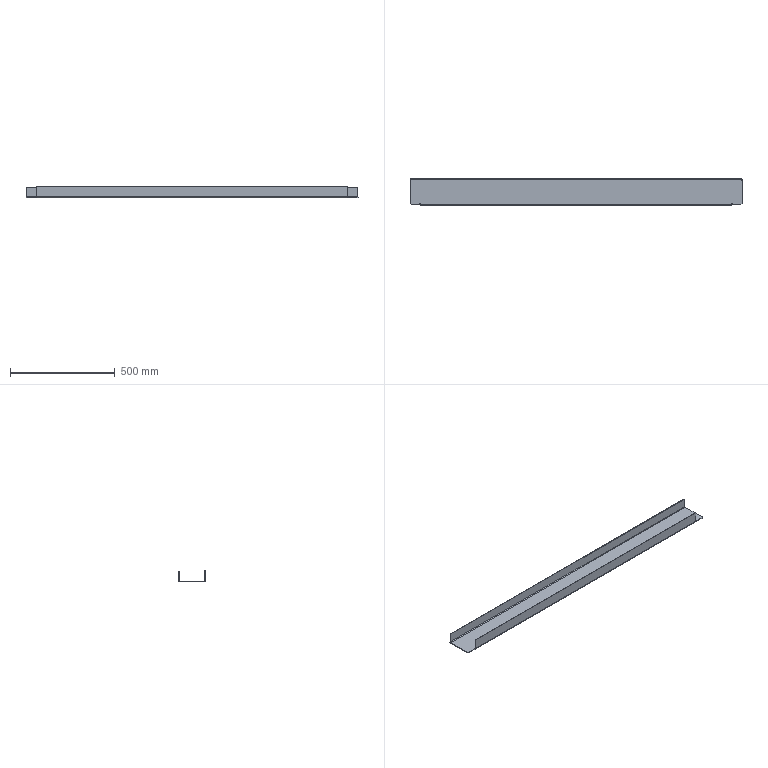Part | STEP file | SYL_0392D6J1SYL0380DJ100-794406 | 1 solid | 40 faces | box 1586 x 127 x 55 mm | volume 1040042 mm3 | plane 34 | cylinder 6 | commonest cylinder face diameters 6 x2 8 x2 12 x2
STEP:
#1=CARTESIAN_POINT('',(-744.,-57.5,3.));
#2=VERTEX_POINT('',#1);
#3=CARTESIAN_POINT('',(-744.,-57.5,0.));
#4=VERTEX_POINT('',#3);
#5=CARTESIAN_POINT('',(-744.,-57.5,0.));
#6=DIRECTION('',(0.,0.,-1.));
#7=VECTOR('',#6,1000.);
#8=LINE('',#5,#7);
#9=EDGE_CURVE('',#2,#4,#8,.T.);
#10=ORIENTED_EDGE('',*,*,#9,.F.);
#11=CARTESIAN_POINT('',(-745.5,-57.5,3.));
#12=VERTEX_POINT('',#11);
#13=CARTESIAN_POINT('',(0.,-57.5,3.));
#14=DIRECTION('',(-1.,0.,0.));
#15=VECTOR('',#14,1000.);
#16=LINE('',#13,#15);
#17=EDGE_CURVE('',#2,#12,#16,.T.);
#18=ORIENTED_EDGE('',*,*,#17,.T.);
#19=CARTESIAN_POINT('',(-745.5,-57.5,0.));
#20=VERTEX_POINT('',#19);
#21=CARTESIAN_POINT('',(-745.5,-57.5,0.));
#22=DIRECTION('',(0.,0.,-1.));
#23=VECTOR('',#22,1000.);
#24=LINE('',#21,#23);
#25=EDGE_CURVE('',#12,#20,#24,.T.);
#26=ORIENTED_EDGE('',*,*,#25,.T.);
#27=CARTESIAN_POINT('',(0.,-57.5,0.));
#28=DIRECTION('',(-1.,0.,0.));
#29=VECTOR('',#28,1000.);
#30=LINE('',#27,#29);
#31=EDGE_CURVE('',#4,#20,#30,.T.);
#32=ORIENTED_EDGE('',*,*,#31,.F.);
#33=EDGE_LOOP('',(#10,#18,#26,#32));
#34=FACE_OUTER_BOUND('',#33,.T.);
#35=CARTESIAN_POINT('',(0.,-57.5,0.));
#36=DIRECTION('',(0.,1.,0.));
#37=DIRECTION('',(-1.,0.,0.));
#38=AXIS2_PLACEMENT_3D('',#35,#36,#37);
#39=PLANE('',#38);
#40=ADVANCED_FACE('',(#34),#39,.F.);
#41=ORIENTED_EDGE('',*,*,#25,.F.);
#42=CARTESIAN_POINT('',(-745.5,-62.,3.));
#43=VERTEX_POINT('',#42);
#44=CARTESIAN_POINT('',(-745.5,0.,3.));
#45=DIRECTION('',(0.,-1.,0.));
#46=VECTOR('',#45,1000.);
#47=LINE('',#44,#46);
#48=EDGE_CURVE('',#12,#43,#47,.T.);
#49=ORIENTED_EDGE('',*,*,#48,.T.);
#50=CARTESIAN_POINT('',(-745.5,-62.,0.));
#51=VERTEX_POINT('',#50);
#52=CARTESIAN_POINT('',(-745.5,-62.,0.));
#53=DIRECTION('',(0.,0.,-1.));
#54=VECTOR('',#53,1000.);
#55=LINE('',#52,#54);
#56=EDGE_CURVE('',#43,#51,#55,.T.);
#57=ORIENTED_EDGE('',*,*,#56,.T.);
#58=CARTESIAN_POINT('',(-745.5,0.,0.));
#59=DIRECTION('',(0.,-1.,0.));
#60=VECTOR('',#59,1000.);
#61=LINE('',#58,#60);
#62=EDGE_CURVE('',#20,#51,#61,.T.);
#63=ORIENTED_EDGE('',*,*,#62,.F.);
#64=EDGE_LOOP('',(#41,#49,#57,#63));
#65=FACE_OUTER_BOUND('',#64,.T.);
#66=CARTESIAN_POINT('',(-745.5,0.,0.));
#67=DIRECTION('',(-1.,0.,0.));
#68=DIRECTION('',(0.,-1.,0.));
#69=AXIS2_PLACEMENT_3D('',#66,#67,#68);
#70=PLANE('',#69);
#71=ADVANCED_FACE('',(#65),#70,.F.);
#72=ORIENTED_EDGE('',*,*,#56,.F.);
#73=CARTESIAN_POINT('',(-788.,-62.,3.));
#74=VERTEX_POINT('',#73);
#75=CARTESIAN_POINT('',(0.,-62.,3.));
#76=DIRECTION('',(1.,0.,0.));
#77=VECTOR('',#76,1000.);
#78=LINE('',#75,#77);
#79=EDGE_CURVE('',#74,#43,#78,.T.);
#80=ORIENTED_EDGE('',*,*,#79,.F.);
#81=CARTESIAN_POINT('',(-788.,-62.,0.));
#82=VERTEX_POINT('',#81);
#83=CARTESIAN_POINT('',(-788.,-62.,0.));
#84=DIRECTION('',(0.,0.,-1.));
#85=VECTOR('',#84,1000.);
#86=LINE('',#83,#85);
#87=EDGE_CURVE('',#74,#82,#86,.T.);
#88=ORIENTED_EDGE('',*,*,#87,.T.);
#89=CARTESIAN_POINT('',(-788.,-62.,0.));
#90=DIRECTION('',(1.,0.,0.));
#91=VECTOR('',#90,1000.);
#92=LINE('',#89,#91);
#93=EDGE_CURVE('',#82,#51,#92,.T.);
#94=ORIENTED_EDGE('',*,*,#93,.T.);
#95=EDGE_LOOP('',(#72,#80,#88,#94));
#96=FACE_OUTER_BOUND('',#95,.T.);
#97=CARTESIAN_POINT('',(-788.,-62.,0.));
#98=DIRECTION('',(0.,-1.,0.));
#99=DIRECTION('',(1.,0.,0.));
#100=AXIS2_PLACEMENT_3D('',#97,#98,#99);
#101=PLANE('',#100);
#102=ADVANCED_FACE('',(#96),#101,.T.);
#103=ORIENTED_EDGE('',*,*,#87,.F.);
#104=CARTESIAN_POINT('',(-793.,-57.,3.));
#105=VERTEX_POINT('',#104);
#106=CARTESIAN_POINT('',(-788.,-62.,3.));
#107=DIRECTION('',(-0.7071,0.7071,0.));
#108=VECTOR('',#107,1000.);
#109=LINE('',#106,#108);
#110=EDGE_CURVE('',#74,#105,#109,.T.);
#111=ORIENTED_EDGE('',*,*,#110,.T.);
#112=CARTESIAN_POINT('',(-793.,-57.,0.));
#113=VERTEX_POINT('',#112);
#114=CARTESIAN_POINT('',(-793.,-57.,0.));
#115=DIRECTION('',(0.,0.,-1.));
#116=VECTOR('',#115,1000.);
#117=LINE('',#114,#116);
#118=EDGE_CURVE('',#105,#113,#117,.T.);
#119=ORIENTED_EDGE('',*,*,#118,.T.);
#120=CARTESIAN_POINT('',(-788.,-62.,0.));
#121=DIRECTION('',(-0.7071,0.7071,0.));
#122=VECTOR('',#121,1000.);
#123=LINE('',#120,#122);
#124=EDGE_CURVE('',#82,#113,#123,.T.);
#125=ORIENTED_EDGE('',*,*,#124,.F.);
#126=EDGE_LOOP('',(#103,#111,#119,#125));
#127=FACE_OUTER_BOUND('',#126,.T.);
#128=CARTESIAN_POINT('',(-788.,-62.,0.));
#129=DIRECTION('',(0.7071,0.7071,0.));
#130=DIRECTION('',(-0.7071,0.7071,0.));
#131=AXIS2_PLACEMENT_3D('',#128,#129,#130);
#132=PLANE('',#131);
#133=ADVANCED_FACE('',(#127),#132,.F.);
#134=ORIENTED_EDGE('',*,*,#118,.F.);
#135=CARTESIAN_POINT('',(-793.,58.,3.));
#136=VERTEX_POINT('',#135);
#137=CARTESIAN_POINT('',(-793.,0.,3.));
#138=DIRECTION('',(0.,-1.,0.));
#139=VECTOR('',#138,1000.);
#140=LINE('',#137,#139);
#141=EDGE_CURVE('',#136,#105,#140,.T.);
#142=ORIENTED_EDGE('',*,*,#141,.F.);
#143=CARTESIAN_POINT('',(-793.,58.,0.));
#144=VERTEX_POINT('',#143);
#145=CARTESIAN_POINT('',(-793.,58.,0.));
#146=DIRECTION('',(0.,0.,-1.));
#147=VECTOR('',#146,1000.);
#148=LINE('',#145,#147);
#149=EDGE_CURVE('',#136,#144,#148,.T.);
#150=ORIENTED_EDGE('',*,*,#149,.T.);
#151=CARTESIAN_POINT('',(-793.,58.,0.));
#152=DIRECTION('',(0.,-1.,0.));
#153=VECTOR('',#152,1000.);
#154=LINE('',#151,#153);
#155=EDGE_CURVE('',#144,#113,#154,.T.);
#156=ORIENTED_EDGE('',*,*,#155,.T.);
#157=EDGE_LOOP('',(#134,#142,#150,#156));
#158=FACE_OUTER_BOUND('',#157,.T.);
#159=CARTESIAN_POINT('',(-793.,58.,0.));
#160=DIRECTION('',(-1.,0.,0.));
#161=DIRECTION('',(0.,-1.,0.));
#162=AXIS2_PLACEMENT_3D('',#159,#160,#161);
#163=PLANE('',#162);
#164=ADVANCED_FACE('',(#158),#163,.T.);
#165=ORIENTED_EDGE('',*,*,#149,.F.);
#166=CARTESIAN_POINT('',(-790.5,61.708,3.));
#167=VERTEX_POINT('',#166);
#168=CARTESIAN_POINT('',(-789.,58.,3.));
#169=DIRECTION('',(0.,0.,-1.));
#170=DIRECTION('',(-1.,0.,0.));
#171=AXIS2_PLACEMENT_3D('',#168,#169,#170);
#172=CIRCLE('',#171,4.);
#173=EDGE_CURVE('',#136,#167,#172,.T.);
#174=ORIENTED_EDGE('',*,*,#173,.T.);
#175=CARTESIAN_POINT('',(-790.5,61.708,0.));
#176=VERTEX_POINT('',#175);
#177=CARTESIAN_POINT('',(-790.5,61.708,0.));
#178=DIRECTION('',(0.,0.,-1.));
#179=VECTOR('',#178,1000.);
#180=LINE('',#177,#179);
#181=EDGE_CURVE('',#167,#176,#180,.T.);
#182=ORIENTED_EDGE('',*,*,#181,.T.);
#183=CARTESIAN_POINT('',(-789.,58.,0.));
#184=DIRECTION('',(0.,0.,-1.));
#185=DIRECTION('',(-1.,0.,0.));
#186=AXIS2_PLACEMENT_3D('',#183,#184,#185);
#187=CIRCLE('',#186,4.);
#188=EDGE_CURVE('',#144,#176,#187,.T.);
#189=ORIENTED_EDGE('',*,*,#188,.F.);
#190=EDGE_LOOP('',(#165,#174,#182,#189));
#191=FACE_OUTER_BOUND('',#190,.T.);
#192=CARTESIAN_POINT('',(-789.,58.,0.));
#193=DIRECTION('',(0.,0.,1.));
#194=DIRECTION('',(1.,0.,0.));
#195=AXIS2_PLACEMENT_3D('',#192,#193,#194);
#196=CYLINDRICAL_SURFACE('',#195,4.);
#197=ADVANCED_FACE('',(#191),#196,.T.);
#198=ORIENTED_EDGE('',*,*,#181,.F.);
#199=CARTESIAN_POINT('',(-790.5,54.5,3.));
#200=VERTEX_POINT('',#199);
#201=CARTESIAN_POINT('',(-790.5,0.,3.));
#202=DIRECTION('',(0.,-1.,0.));
#203=VECTOR('',#202,1000.);
#204=LINE('',#201,#203);
#205=EDGE_CURVE('',#167,#200,#204,.T.);
#206=ORIENTED_EDGE('',*,*,#205,.T.);
#207=CARTESIAN_POINT('',(-790.5,54.5,0.));
#208=VERTEX_POINT('',#207);
#209=CARTESIAN_POINT('',(-790.5,54.5,0.));
#210=DIRECTION('',(0.,0.,-1.));
#211=VECTOR('',#210,1000.);
#212=LINE('',#209,#211);
#213=EDGE_CURVE('',#200,#208,#212,.T.);
#214=ORIENTED_EDGE('',*,*,#213,.T.);
#215=CARTESIAN_POINT('',(-790.5,0.,0.));
#216=DIRECTION('',(0.,-1.,0.));
#217=VECTOR('',#216,1000.);
#218=LINE('',#215,#217);
#219=EDGE_CURVE('',#176,#208,#218,.T.);
#220=ORIENTED_EDGE('',*,*,#219,.F.);
#221=EDGE_LOOP('',(#198,#206,#214,#220));
#222=FACE_OUTER_BOUND('',#221,.T.);
#223=CARTESIAN_POINT('',(-790.5,0.,0.));
#224=DIRECTION('',(-1.,0.,0.));
#225=DIRECTION('',(0.,-1.,0.));
#226=AXIS2_PLACEMENT_3D('',#223,#224,#225);
#227=PLANE('',#226);
#228=ADVANCED_FACE('',(#222),#227,.F.);
#229=ORIENTED_EDGE('',*,*,#213,.F.);
#230=CARTESIAN_POINT('',(-789.,54.5,3.));
#231=VERTEX_POINT('',#230);
#232=CARTESIAN_POINT('',(0.,54.5,3.));
#233=DIRECTION('',(1.,0.,0.));
#234=VECTOR('',#233,1000.);
#235=LINE('',#232,#234);
#236=EDGE_CURVE('',#200,#231,#235,.T.);
#237=ORIENTED_EDGE('',*,*,#236,.T.);
#238=CARTESIAN_POINT('',(-789.,54.5,0.));
#239=VERTEX_POINT('',#238);
#240=CARTESIAN_POINT('',(-789.,54.5,0.));
#241=DIRECTION('',(0.,0.,-1.));
#242=VECTOR('',#241,1000.);
#243=LINE('',#240,#242);
#244=EDGE_CURVE('',#231,#239,#243,.T.);
#245=ORIENTED_EDGE('',*,*,#244,.T.);
#246=CARTESIAN_POINT('',(0.,54.5,0.));
#247=DIRECTION('',(1.,0.,0.));
#248=VECTOR('',#247,1000.);
#249=LINE('',#246,#248);
#250=EDGE_CURVE('',#208,#239,#249,.T.);
#251=ORIENTED_EDGE('',*,*,#250,.F.);
#252=EDGE_LOOP('',(#229,#237,#245,#251));
#253=FACE_OUTER_BOUND('',#252,.T.);
#254=CARTESIAN_POINT('',(0.,54.5,0.));
#255=DIRECTION('',(0.,-1.,0.));
#256=DIRECTION('',(1.,0.,0.));
#257=AXIS2_PLACEMENT_3D('',#254,#255,#256);
#258=PLANE('',#257);
#259=ADVANCED_FACE('',(#253),#258,.F.);
#260=ORIENTED_EDGE('',*,*,#244,.F.);
#261=CARTESIAN_POINT('',(-789.,56.,3.));
#262=VERTEX_POINT('',#261);
#263=CARTESIAN_POINT('',(-789.,0.,3.));
#264=DIRECTION('',(0.,1.,0.));
#265=VECTOR('',#264,1000.);
#266=LINE('',#263,#265);
#267=EDGE_CURVE('',#231,#262,#266,.T.);
#268=ORIENTED_EDGE('',*,*,#267,.T.);
#269=CARTESIAN_POINT('',(-789.,56.,0.));
#270=VERTEX_POINT('',#269);
#271=CARTESIAN_POINT('',(-789.,56.,0.));
#272=DIRECTION('',(0.,0.,-1.));
#273=VECTOR('',#272,1000.);
#274=LINE('',#271,#273);
#275=EDGE_CURVE('',#262,#270,#274,.T.);
#276=ORIENTED_EDGE('',*,*,#275,.T.);
#277=CARTESIAN_POINT('',(-789.,0.,0.));
#278=DIRECTION('',(0.,1.,0.));
#279=VECTOR('',#278,1000.);
#280=LINE('',#277,#279);
#281=EDGE_CURVE('',#239,#270,#280,.T.);
#282=ORIENTED_EDGE('',*,*,#281,.F.);
#283=EDGE_LOOP('',(#260,#268,#276,#282));
#284=FACE_OUTER_BOUND('',#283,.T.);
#285=CARTESIAN_POINT('',(-789.,0.,0.));
#286=DIRECTION('',(1.,0.,0.));
#287=DIRECTION('',(0.,1.,0.));
#288=AXIS2_PLACEMENT_3D('',#285,#286,#287);
#289=PLANE('',#288);
#290=ADVANCED_FACE('',(#284),#289,.F.);
#291=ORIENTED_EDGE('',*,*,#275,.F.);
#292=CARTESIAN_POINT('',(-789.,59.,6.));
#293=VERTEX_POINT('',#292);
#294=CARTESIAN_POINT('',(-789.,56.,6.));
#295=DIRECTION('',(-1.,0.,0.));
#296=DIRECTION('',(0.,0.,1.));
#297=AXIS2_PLACEMENT_3D('',#294,#295,#296);
#298=CIRCLE('',#297,3.);
#299=EDGE_CURVE('',#293,#262,#298,.T.);
#300=ORIENTED_EDGE('',*,*,#299,.F.);
#301=CARTESIAN_POINT('',(-789.,62.,6.));
#302=VERTEX_POINT('',#301);
#303=CARTESIAN_POINT('',(-789.,62.,6.));
#304=DIRECTION('',(0.,1.,0.));
#305=VECTOR('',#304,1000.);
#306=LINE('',#303,#305);
#307=EDGE_CURVE('',#293,#302,#306,.T.);
#308=ORIENTED_EDGE('',*,*,#307,.T.);
#309=CARTESIAN_POINT('',(-789.,56.,6.));
#310=DIRECTION('',(-1.,0.,0.));
#311=DIRECTION('',(0.,1.,0.));
#312=AXIS2_PLACEMENT_3D('',#309,#310,#311);
#313=CIRCLE('',#312,6.);
#314=EDGE_CURVE('',#302,#270,#313,.T.);
#315=ORIENTED_EDGE('',*,*,#314,.T.);
#316=EDGE_LOOP('',(#291,#300,#308,#315));
#317=FACE_OUTER_BOUND('',#316,.T.);
#318=CARTESIAN_POINT('',(-789.,56.,6.));
#319=DIRECTION('',(1.,0.,0.));
#320=DIRECTION('',(0.,0.,-1.));
#321=AXIS2_PLACEMENT_3D('',#318,#319,#320);
#322=PLANE('',#321);
#323=ADVANCED_FACE('',(#317),#322,.F.);
#324=ORIENTED_EDGE('',*,*,#307,.F.);
#325=CARTESIAN_POINT('',(-789.,59.,50.));
#326=VERTEX_POINT('',#325);
#327=CARTESIAN_POINT('',(-789.,59.,0.));
#328=DIRECTION('',(0.,0.,1.));
#329=VECTOR('',#328,1000.);
#330=LINE('',#327,#329);
#331=EDGE_CURVE('',#293,#326,#330,.T.);
#332=ORIENTED_EDGE('',*,*,#331,.T.);
#333=CARTESIAN_POINT('',(-789.,62.,50.));
#334=VERTEX_POINT('',#333);
#335=CARTESIAN_POINT('',(-789.,62.,50.));
#336=DIRECTION('',(0.,1.,0.));
#337=VECTOR('',#336,1000.);
#338=LINE('',#335,#337);
#339=EDGE_CURVE('',#326,#334,#338,.T.);
#340=ORIENTED_EDGE('',*,*,#339,.T.);
#341=CARTESIAN_POINT('',(-789.,62.,6.));
#342=DIRECTION('',(0.,0.,1.));
#343=VECTOR('',#342,1000.);
#344=LINE('',#341,#343);
#345=EDGE_CURVE('',#302,#334,#344,.T.);
#346=ORIENTED_EDGE('',*,*,#345,.F.);
#347=EDGE_LOOP('',(#324,#332,#340,#346));
#348=FACE_OUTER_BOUND('',#347,.T.);
#349=CARTESIAN_POINT('',(-789.,62.,6.));
#350=DIRECTION('',(-1.,0.,0.));
#351=DIRECTION('',(0.,0.,1.));
#352=AXIS2_PLACEMENT_3D('',#349,#350,#351);
#353=PLANE('',#352);
#354=ADVANCED_FACE('',(#348),#353,.T.);
#355=ORIENTED_EDGE('',*,*,#339,.F.);
#356=CARTESIAN_POINT('',(789.,59.,50.));
#357=VERTEX_POINT('',#356);
#358=CARTESIAN_POINT('',(-789.,59.,50.));
#359=DIRECTION('',(1.,0.,0.));
#360=VECTOR('',#359,1000.);
#361=LINE('',#358,#360);
#362=EDGE_CURVE('',#326,#357,#361,.T.);
#363=ORIENTED_EDGE('',*,*,#362,.T.);
#364=CARTESIAN_POINT('',(789.,62.,50.));
#365=VERTEX_POINT('',#364);
#366=CARTESIAN_POINT('',(789.,62.,50.));
#367=DIRECTION('',(0.,1.,0.));
#368=VECTOR('',#367,1000.);
#369=LINE('',#366,#368);
#370=EDGE_CURVE('',#357,#365,#369,.T.);
#371=ORIENTED_EDGE('',*,*,#370,.T.);
#372=CARTESIAN_POINT('',(-789.,62.,50.));
#373=DIRECTION('',(1.,0.,0.));
#374=VECTOR('',#373,1000.);
#375=LINE('',#372,#374);
#376=EDGE_CURVE('',#334,#365,#375,.T.);
#377=ORIENTED_EDGE('',*,*,#376,.F.);
#378=EDGE_LOOP('',(#355,#363,#371,#377));
#379=FACE_OUTER_BOUND('',#378,.T.);
#380=CARTESIAN_POINT('',(-789.,62.,50.));
#381=DIRECTION('',(0.,0.,1.));
#382=DIRECTION('',(1.,0.,0.));
#383=AXIS2_PLACEMENT_3D('',#380,#381,#382);
#384=PLANE('',#383);
#385=ADVANCED_FACE('',(#379),#384,.T.);
#386=ORIENTED_EDGE('',*,*,#370,.F.);
#387=CARTESIAN_POINT('',(789.,59.,6.));
#388=VERTEX_POINT('',#387);
#389=CARTESIAN_POINT('',(789.,59.,0.));
#390=DIRECTION('',(0.,0.,-1.));
#391=VECTOR('',#390,1000.);
#392=LINE('',#389,#391);
#393=EDGE_CURVE('',#357,#388,#392,.T.);
#394=ORIENTED_EDGE('',*,*,#393,.T.);
#395=CARTESIAN_POINT('',(789.,62.,6.));
#396=VERTEX_POINT('',#395);
#397=CARTESIAN_POINT('',(789.,62.,6.));
#398=DIRECTION('',(0.,1.,0.));
#399=VECTOR('',#398,1000.);
#400=LINE('',#397,#399);
#401=EDGE_CURVE('',#388,#396,#400,.T.);
#402=ORIENTED_EDGE('',*,*,#401,.T.);
#403=CARTESIAN_POINT('',(789.,62.,50.));
#404=DIRECTION('',(0.,0.,-1.));
#405=VECTOR('',#404,1000.);
#406=LINE('',#403,#405);
#407=EDGE_CURVE('',#365,#396,#406,.T.);
#408=ORIENTED_EDGE('',*,*,#407,.F.);
#409=EDGE_LOOP('',(#386,#394,#402,#408));
#410=FACE_OUTER_BOUND('',#409,.T.);
#411=CARTESIAN_POINT('',(789.,62.,50.));
#412=DIRECTION('',(1.,0.,0.));
#413=DIRECTION('',(0.,0.,-1.));
#414=AXIS2_PLACEMENT_3D('',#411,#412,#413);
#415=PLANE('',#414);
#416=ADVANCED_FACE('',(#410),#415,.T.);
#417=ORIENTED_EDGE('',*,*,#401,.F.);
#418=CARTESIAN_POINT('',(789.,56.,3.));
#419=VERTEX_POINT('',#418);
#420=CARTESIAN_POINT('',(789.,56.,6.));
#421=DIRECTION('',(1.,0.,0.));
#422=DIRECTION('',(0.,0.,1.));
#423=AXIS2_PLACEMENT_3D('',#420,#421,#422);
#424=CIRCLE('',#423,3.);
#425=EDGE_CURVE('',#419,#388,#424,.T.);
#426=ORIENTED_EDGE('',*,*,#425,.F.);
#427=CARTESIAN_POINT('',(789.,56.,0.));
#428=VERTEX_POINT('',#427);
#429=CARTESIAN_POINT('',(789.,56.,0.));
#430=DIRECTION('',(0.,0.,-1.));
#431=VECTOR('',#430,1000.);
#432=LINE('',#429,#431);
#433=EDGE_CURVE('',#419,#428,#432,.T.);
#434=ORIENTED_EDGE('',*,*,#433,.T.);
#435=CARTESIAN_POINT('',(789.,56.,6.));
#436=DIRECTION('',(1.,0.,0.));
#437=DIRECTION('',(0.,0.,-1.));
#438=AXIS2_PLACEMENT_3D('',#435,#436,#437);
#439=CIRCLE('',#438,6.);
#440=EDGE_CURVE('',#428,#396,#439,.T.);
#441=ORIENTED_EDGE('',*,*,#440,.T.);
#442=EDGE_LOOP('',(#417,#426,#434,#441));
#443=FACE_OUTER_BOUND('',#442,.T.);
#444=CARTESIAN_POINT('',(789.,56.,6.));
#445=DIRECTION('',(-1.,0.,0.));
#446=DIRECTION('',(0.,0.,1.));
#447=AXIS2_PLACEMENT_3D('',#444,#445,#446);
#448=PLANE('',#447);
#449=ADVANCED_FACE('',(#443),#448,.F.);
#450=ORIENTED_EDGE('',*,*,#433,.F.);
#451=CARTESIAN_POINT('',(789.,54.5,3.));
#452=VERTEX_POINT('',#451);
#453=CARTESIAN_POINT('',(789.,0.,3.));
#454=DIRECTION('',(0.,-1.,0.));
#455=VECTOR('',#454,1000.);
#456=LINE('',#453,#455);
#457=EDGE_CURVE('',#419,#452,#456,.T.);
#458=ORIENTED_EDGE('',*,*,#457,.T.);
#459=CARTESIAN_POINT('',(789.,54.5,0.));
#460=VERTEX_POINT('',#459);
#461=CARTESIAN_POINT('',(789.,54.5,0.));
#462=DIRECTION('',(0.,0.,-1.));
#463=VECTOR('',#462,1000.);
#464=LINE('',#461,#463);
#465=EDGE_CURVE('',#452,#460,#464,.T.);
#466=ORIENTED_EDGE('',*,*,#465,.T.);
#467=CARTESIAN_POINT('',(789.,0.,0.));
#468=DIRECTION('',(0.,-1.,0.));
#469=VECTOR('',#468,1000.);
#470=LINE('',#467,#469);
#471=EDGE_CURVE('',#428,#460,#470,.T.);
#472=ORIENTED_EDGE('',*,*,#471,.F.);
#473=EDGE_LOOP('',(#450,#458,#466,#472));
#474=FACE_OUTER_BOUND('',#473,.T.);
#475=CARTESIAN_POINT('',(789.,0.,0.));
#476=DIRECTION('',(-1.,0.,0.));
#477=DIRECTION('',(0.,-1.,0.));
#478=AXIS2_PLACEMENT_3D('',#475,#476,#477);
#479=PLANE('',#478);
#480=ADVANCED_FACE('',(#474),#479,.F.);
#481=ORIENTED_EDGE('',*,*,#465,.F.);
#482=CARTESIAN_POINT('',(790.5,54.5,3.));
#483=VERTEX_POINT('',#482);
#484=CARTESIAN_POINT('',(0.,54.5,3.));
#485=DIRECTION('',(1.,0.,0.));
#486=VECTOR('',#485,1000.);
#487=LINE('',#484,#486);
#488=EDGE_CURVE('',#452,#483,#487,.T.);
#489=ORIENTED_EDGE('',*,*,#488,.T.);
#490=CARTESIAN_POINT('',(790.5,54.5,0.));
#491=VERTEX_POINT('',#490);
#492=CARTESIAN_POINT('',(790.5,54.5,0.));
#493=DIRECTION('',(0.,0.,-1.));
#494=VECTOR('',#493,1000.);
#495=LINE('',#492,#494);
#496=EDGE_CURVE('',#483,#491,#495,.T.);
#497=ORIENTED_EDGE('',*,*,#496,.T.);
#498=CARTESIAN_POINT('',(0.,54.5,0.));
#499=DIRECTION('',(1.,0.,0.));
#500=VECTOR('',#499,1000.);
#501=LINE('',#498,#500);
#502=EDGE_CURVE('',#460,#491,#501,.T.);
#503=ORIENTED_EDGE('',*,*,#502,.F.);
#504=EDGE_LOOP('',(#481,#489,#497,#503));
#505=FACE_OUTER_BOUND('',#504,.T.);
#506=CARTESIAN_POINT('',(0.,54.5,0.));
#507=DIRECTION('',(0.,-1.,0.));
#508=DIRECTION('',(1.,0.,0.));
#509=AXIS2_PLACEMENT_3D('',#506,#507,#508);
#510=PLANE('',#509);
#511=ADVANCED_FACE('',(#505),#510,.F.);
#512=ORIENTED_EDGE('',*,*,#496,.F.);
#513=CARTESIAN_POINT('',(790.5,61.708,3.));
#514=VERTEX_POINT('',#513);
#515=CARTESIAN_POINT('',(790.5,0.,3.));
#516=DIRECTION('',(0.,1.,0.));
#517=VECTOR('',#516,1000.);
#518=LINE('',#515,#517);
#519=EDGE_CURVE('',#483,#514,#518,.T.);
#520=ORIENTED_EDGE('',*,*,#519,.T.);
#521=CARTESIAN_POINT('',(790.5,61.708,0.));
#522=VERTEX_POINT('',#521);
#523=CARTESIAN_POINT('',(790.5,61.708,0.));
#524=DIRECTION('',(0.,0.,-1.));
#525=VECTOR('',#524,1000.);
#526=LINE('',#523,#525);
#527=EDGE_CURVE('',#514,#522,#526,.T.);
#528=ORIENTED_EDGE('',*,*,#527,.T.);
#529=CARTESIAN_POINT('',(790.5,0.,0.));
#530=DIRECTION('',(0.,1.,0.));
#531=VECTOR('',#530,1000.);
#532=LINE('',#529,#531);
#533=EDGE_CURVE('',#491,#522,#532,.T.);
#534=ORIENTED_EDGE('',*,*,#533,.F.);
#535=EDGE_LOOP('',(#512,#520,#528,#534));
#536=FACE_OUTER_BOUND('',#535,.T.);
#537=CARTESIAN_POINT('',(790.5,0.,0.));
#538=DIRECTION('',(1.,0.,0.));
#539=DIRECTION('',(0.,1.,0.));
#540=AXIS2_PLACEMENT_3D('',#537,#538,#539);
#541=PLANE('',#540);
#542=ADVANCED_FACE('',(#536),#541,.F.);
#543=ORIENTED_EDGE('',*,*,#527,.F.);
#544=CARTESIAN_POINT('',(793.,58.,3.));
#545=VERTEX_POINT('',#544);
#546=CARTESIAN_POINT('',(789.,58.,3.));
#547=DIRECTION('',(0.,0.,-1.));
#548=DIRECTION('',(-1.,0.,0.));
#549=AXIS2_PLACEMENT_3D('',#546,#547,#548);
#550=CIRCLE('',#549,4.);
#551=EDGE_CURVE('',#514,#545,#550,.T.);
#552=ORIENTED_EDGE('',*,*,#551,.T.);
#553=CARTESIAN_POINT('',(793.,58.,0.));
#554=VERTEX_POINT('',#553);
#555=CARTESIAN_POINT('',(793.,58.,0.));
#556=DIRECTION('',(0.,0.,-1.));
#557=VECTOR('',#556,1000.);
#558=LINE('',#555,#557);
#559=EDGE_CURVE('',#545,#554,#558,.T.);
#560=ORIENTED_EDGE('',*,*,#559,.T.);
#561=CARTESIAN_POINT('',(789.,58.,0.));
#562=DIRECTION('',(0.,0.,-1.));
#563=DIRECTION('',(0.,1.,0.));
#564=AXIS2_PLACEMENT_3D('',#561,#562,#563);
#565=CIRCLE('',#564,4.);
#566=EDGE_CURVE('',#522,#554,#565,.T.);
#567=ORIENTED_EDGE('',*,*,#566,.F.);
#568=EDGE_LOOP('',(#543,#552,#560,#567));
#569=FACE_OUTER_BOUND('',#568,.T.);
#570=CARTESIAN_POINT('',(789.,58.,0.));
#571=DIRECTION('',(0.,0.,1.));
#572=DIRECTION('',(1.,0.,0.));
#573=AXIS2_PLACEMENT_3D('',#570,#571,#572);
#574=CYLINDRICAL_SURFACE('',#573,4.);
#575=ADVANCED_FACE('',(#569),#574,.T.);
#576=ORIENTED_EDGE('',*,*,#559,.F.);
#577=CARTESIAN_POINT('',(793.,-57.,3.));
#578=VERTEX_POINT('',#577);
#579=CARTESIAN_POINT('',(793.,0.,3.));
#580=DIRECTION('',(0.,1.,0.));
#581=VECTOR('',#580,1000.);
#582=LINE('',#579,#581);
#583=EDGE_CURVE('',#578,#545,#582,.T.);
#584=ORIENTED_EDGE('',*,*,#583,.F.);
#585=CARTESIAN_POINT('',(793.,-57.,0.));
#586=VERTEX_POINT('',#585);
#587=CARTESIAN_POINT('',(793.,-57.,0.));
#588=DIRECTION('',(0.,0.,-1.));
#589=VECTOR('',#588,1000.);
#590=LINE('',#587,#589);
#591=EDGE_CURVE('',#578,#586,#590,.T.);
#592=ORIENTED_EDGE('',*,*,#591,.T.);
#593=CARTESIAN_POINT('',(793.,-57.,0.));
#594=DIRECTION('',(0.,1.,0.));
#595=VECTOR('',#594,1000.);
#596=LINE('',#593,#595);
#597=EDGE_CURVE('',#586,#554,#596,.T.);
#598=ORIENTED_EDGE('',*,*,#597,.T.);
#599=EDGE_LOOP('',(#576,#584,#592,#598));
#600=FACE_OUTER_BOUND('',#599,.T.);
#601=CARTESIAN_POINT('',(793.,-57.,0.));
#602=DIRECTION('',(1.,0.,0.));
#603=DIRECTION('',(0.,1.,0.));
#604=AXIS2_PLACEMENT_3D('',#601,#602,#603);
#605=PLANE('',#604);
#606=ADVANCED_FACE('',(#600),#605,.T.);
#607=ORIENTED_EDGE('',*,*,#591,.F.);
#608=CARTESIAN_POINT('',(788.,-62.,3.));
#609=VERTEX_POINT('',#608);
#610=CARTESIAN_POINT('',(793.,-57.,3.));
#611=DIRECTION('',(-0.7071,-0.7071,0.));
#612=VECTOR('',#611,1000.);
#613=LINE('',#610,#612);
#614=EDGE_CURVE('',#578,#609,#613,.T.);
#615=ORIENTED_EDGE('',*,*,#614,.T.);
#616=CARTESIAN_POINT('',(788.,-62.,0.));
#617=VERTEX_POINT('',#616);
#618=CARTESIAN_POINT('',(788.,-62.,0.));
#619=DIRECTION('',(0.,0.,-1.));
#620=VECTOR('',#619,1000.);
#621=LINE('',#618,#620);
#622=EDGE_CURVE('',#609,#617,#621,.T.);
#623=ORIENTED_EDGE('',*,*,#622,.T.);
#624=CARTESIAN_POINT('',(793.,-57.,0.));
#625=DIRECTION('',(-0.7071,-0.7071,0.));
#626=VECTOR('',#625,1000.);
#627=LINE('',#624,#626);
#628=EDGE_CURVE('',#586,#617,#627,.T.);
#629=ORIENTED_EDGE('',*,*,#628,.F.);
#630=EDGE_LOOP('',(#607,#615,#623,#629));
#631=FACE_OUTER_BOUND('',#630,.T.);
#632=CARTESIAN_POINT('',(793.,-57.,0.));
#633=DIRECTION('',(-0.7071,0.7071,0.));
#634=DIRECTION('',(-0.7071,-0.7071,0.));
#635=AXIS2_PLACEMENT_3D('',#632,#633,#634);
#636=PLANE('',#635);
#637=ADVANCED_FACE('',(#631),#636,.F.);
#638=ORIENTED_EDGE('',*,*,#622,.F.);
#639=CARTESIAN_POINT('',(745.5,-62.,3.));
#640=VERTEX_POINT('',#639);
#641=CARTESIAN_POINT('',(0.,-62.,3.));
#642=DIRECTION('',(1.,0.,0.));
#643=VECTOR('',#642,1000.);
#644=LINE('',#641,#643);
#645=EDGE_CURVE('',#640,#609,#644,.T.);
#646=ORIENTED_EDGE('',*,*,#645,.F.);
#647=CARTESIAN_POINT('',(745.5,-62.,0.));
#648=VERTEX_POINT('',#647);
#649=CARTESIAN_POINT('',(745.5,-62.,0.));
#650=DIRECTION('',(0.,0.,-1.));
#651=VECTOR('',#650,1000.);
#652=LINE('',#649,#651);
#653=EDGE_CURVE('',#640,#648,#652,.T.);
#654=ORIENTED_EDGE('',*,*,#653,.T.);
#655=CARTESIAN_POINT('',(744.,-62.,0.));
#656=DIRECTION('',(1.,0.,0.));
#657=VECTOR('',#656,1000.);
#658=LINE('',#655,#657);
#659=EDGE_CURVE('',#648,#617,#658,.T.);
#660=ORIENTED_EDGE('',*,*,#659,.T.);
#661=EDGE_LOOP('',(#638,#646,#654,#660));
#662=FACE_OUTER_BOUND('',#661,.T.);
#663=CARTESIAN_POINT('',(744.,-62.,0.));
#664=DIRECTION('',(0.,-1.,0.));
#665=DIRECTION('',(1.,0.,0.));
#666=AXIS2_PLACEMENT_3D('',#663,#664,#665);
#667=PLANE('',#666);
#668=ADVANCED_FACE('',(#662),#667,.T.);
#669=ORIENTED_EDGE('',*,*,#653,.F.);
#670=CARTESIAN_POINT('',(745.5,-57.5,3.));
#671=VERTEX_POINT('',#670);
#672=CARTESIAN_POINT('',(745.5,0.,3.));
#673=DIRECTION('',(0.,1.,0.));
#674=VECTOR('',#673,1000.);
#675=LINE('',#672,#674);
#676=EDGE_CURVE('',#640,#671,#675,.T.);
#677=ORIENTED_EDGE('',*,*,#676,.T.);
#678=CARTESIAN_POINT('',(745.5,-57.5,0.));
#679=VERTEX_POINT('',#678);
#680=CARTESIAN_POINT('',(745.5,-57.5,0.));
#681=DIRECTION('',(0.,0.,-1.));
#682=VECTOR('',#681,1000.);
#683=LINE('',#680,#682);
#684=EDGE_CURVE('',#671,#679,#683,.T.);
#685=ORIENTED_EDGE('',*,*,#684,.T.);
#686=CARTESIAN_POINT('',(745.5,0.,0.));
#687=DIRECTION('',(0.,1.,0.));
#688=VECTOR('',#687,1000.);
#689=LINE('',#686,#688);
#690=EDGE_CURVE('',#648,#679,#689,.T.);
#691=ORIENTED_EDGE('',*,*,#690,.F.);
#692=EDGE_LOOP('',(#669,#677,#685,#691));
#693=FACE_OUTER_BOUND('',#692,.T.);
#694=CARTESIAN_POINT('',(745.5,0.,0.));
#695=DIRECTION('',(1.,0.,0.));
#696=DIRECTION('',(0.,1.,0.));
#697=AXIS2_PLACEMENT_3D('',#694,#695,#696);
#698=PLANE('',#697);
#699=ADVANCED_FACE('',(#693),#698,.F.);
#700=ORIENTED_EDGE('',*,*,#684,.F.);
#701=CARTESIAN_POINT('',(744.,-57.5,3.));
#702=VERTEX_POINT('',#701);
#703=CARTESIAN_POINT('',(0.,-57.5,3.));
#704=DIRECTION('',(-1.,0.,0.));
#705=VECTOR('',#704,1000.);
#706=LINE('',#703,#705);
#707=EDGE_CURVE('',#671,#702,#706,.T.);
#708=ORIENTED_EDGE('',*,*,#707,.T.);
#709=CARTESIAN_POINT('',(744.,-57.5,0.));
#710=VERTEX_POINT('',#709);
#711=CARTESIAN_POINT('',(744.,-57.5,0.));
#712=DIRECTION('',(0.,0.,-1.));
#713=VECTOR('',#712,1000.);
#714=LINE('',#711,#713);
#715=EDGE_CURVE('',#702,#710,#714,.T.);
#716=ORIENTED_EDGE('',*,*,#715,.T.);
#717=CARTESIAN_POINT('',(0.,-57.5,0.));
#718=DIRECTION('',(-1.,0.,0.));
#719=VECTOR('',#718,1000.);
#720=LINE('',#717,#719);
#721=EDGE_CURVE('',#679,#710,#720,.T.);
#722=ORIENTED_EDGE('',*,*,#721,.F.);
#723=EDGE_LOOP('',(#700,#708,#716,#722));
#724=FACE_OUTER_BOUND('',#723,.T.);
#725=CARTESIAN_POINT('',(0.,-57.5,0.));
#726=DIRECTION('',(0.,1.,0.));
#727=DIRECTION('',(-1.,0.,0.));
#728=AXIS2_PLACEMENT_3D('',#725,#726,#727);
#729=PLANE('',#728);
#730=ADVANCED_FACE('',(#724),#729,.F.);
#731=ORIENTED_EDGE('',*,*,#715,.F.);
#732=CARTESIAN_POINT('',(744.,-59.,3.));
#733=VERTEX_POINT('',#732);
#734=CARTESIAN_POINT('',(744.,0.,3.));
#735=DIRECTION('',(0.,-1.,0.));
#736=VECTOR('',#735,1000.);
#737=LINE('',#734,#736);
#738=EDGE_CURVE('',#702,#733,#737,.T.);
#739=ORIENTED_EDGE('',*,*,#738,.T.);
#740=CARTESIAN_POINT('',(744.,-59.,0.));
#741=VERTEX_POINT('',#740);
#742=CARTESIAN_POINT('',(744.,-59.,0.));
#743=DIRECTION('',(0.,0.,-1.));
#744=VECTOR('',#743,1000.);
#745=LINE('',#742,#744);
#746=EDGE_CURVE('',#733,#741,#745,.T.);
#747=ORIENTED_EDGE('',*,*,#746,.T.);
#748=CARTESIAN_POINT('',(744.,0.,0.));
#749=DIRECTION('',(0.,-1.,0.));
#750=VECTOR('',#749,1000.);
#751=LINE('',#748,#750);
#752=EDGE_CURVE('',#710,#741,#751,.T.);
#753=ORIENTED_EDGE('',*,*,#752,.F.);
#754=EDGE_LOOP('',(#731,#739,#747,#753));
#755=FACE_OUTER_BOUND('',#754,.T.);
#756=CARTESIAN_POINT('',(744.,0.,0.));
#757=DIRECTION('',(-1.,0.,0.));
#758=DIRECTION('',(0.,-1.,0.));
#759=AXIS2_PLACEMENT_3D('',#756,#757,#758);
#760=PLANE('',#759);
#761=ADVANCED_FACE('',(#755),#760,.F.);
#762=ORIENTED_EDGE('',*,*,#746,.F.);
#763=CARTESIAN_POINT('',(744.,-62.,6.));
#764=VERTEX_POINT('',#763);
#765=CARTESIAN_POINT('',(744.,-59.,6.));
#766=DIRECTION('',(1.,0.,0.));
#767=DIRECTION('',(0.,0.,-1.));
#768=AXIS2_PLACEMENT_3D('',#765,#766,#767);
#769=CIRCLE('',#768,3.);
#770=EDGE_CURVE('',#764,#733,#769,.T.);
#771=ORIENTED_EDGE('',*,*,#770,.F.);
#772=CARTESIAN_POINT('',(744.,-65.,6.));
#773=VERTEX_POINT('',#772);
#774=CARTESIAN_POINT('',(744.,-65.,6.));
#775=DIRECTION('',(0.,-1.,0.));
#776=VECTOR('',#775,1000.);
#777=LINE('',#774,#776);
#778=EDGE_CURVE('',#764,#773,#777,.T.);
#779=ORIENTED_EDGE('',*,*,#778,.T.);
#780=CARTESIAN_POINT('',(744.,-59.,6.));
#781=DIRECTION('',(1.,0.,0.));
#782=DIRECTION('',(0.,-1.,0.));
#783=AXIS2_PLACEMENT_3D('',#780,#781,#782);
#784=CIRCLE('',#783,6.);
#785=EDGE_CURVE('',#773,#741,#784,.T.);
#786=ORIENTED_EDGE('',*,*,#785,.T.);
#787=EDGE_LOOP('',(#762,#771,#779,#786));
#788=FACE_OUTER_BOUND('',#787,.T.);
#789=CARTESIAN_POINT('',(744.,-59.,6.));
#790=DIRECTION('',(-1.,0.,0.));
#791=DIRECTION('',(0.,0.,1.));
#792=AXIS2_PLACEMENT_3D('',#789,#790,#791);
#793=PLANE('',#792);
#794=ADVANCED_FACE('',(#788),#793,.F.);
#795=ORIENTED_EDGE('',*,*,#778,.F.);
#796=CARTESIAN_POINT('',(744.,-62.,55.));
#797=VERTEX_POINT('',#796);
#798=CARTESIAN_POINT('',(744.,-62.,0.));
#799=DIRECTION('',(0.,0.,1.));
#800=VECTOR('',#799,1000.);
#801=LINE('',#798,#800);
#802=EDGE_CURVE('',#764,#797,#801,.T.);
#803=ORIENTED_EDGE('',*,*,#802,.T.);
#804=CARTESIAN_POINT('',(744.,-65.,55.));
#805=VERTEX_POINT('',#804);
#806=CARTESIAN_POINT('',(744.,-65.,55.));
#807=DIRECTION('',(0.,-1.,0.));
#808=VECTOR('',#807,1000.);
#809=LINE('',#806,#808);
#810=EDGE_CURVE('',#797,#805,#809,.T.);
#811=ORIENTED_EDGE('',*,*,#810,.T.);
#812=CARTESIAN_POINT('',(744.,-65.,6.));
#813=DIRECTION('',(0.,0.,1.));
#814=VECTOR('',#813,1000.);
#815=LINE('',#812,#814);
#816=EDGE_CURVE('',#773,#805,#815,.T.);
#817=ORIENTED_EDGE('',*,*,#816,.F.);
#818=EDGE_LOOP('',(#795,#803,#811,#817));
#819=FACE_OUTER_BOUND('',#818,.T.);
#820=CARTESIAN_POINT('',(744.,-65.,6.));
#821=DIRECTION('',(1.,0.,0.));
#822=DIRECTION('',(0.,0.,1.));
#823=AXIS2_PLACEMENT_3D('',#820,#821,#822);
#824=PLANE('',#823);
#825=ADVANCED_FACE('',(#819),#824,.T.);
#826=ORIENTED_EDGE('',*,*,#810,.F.);
#827=CARTESIAN_POINT('',(-744.,-62.,55.));
#828=VERTEX_POINT('',#827);
#829=CARTESIAN_POINT('',(-416.166,-62.,55.));
#830=DIRECTION('',(-1.,0.,0.));
#831=VECTOR('',#830,1000.);
#832=LINE('',#829,#831);
#833=EDGE_CURVE('',#797,#828,#832,.T.);
#834=ORIENTED_EDGE('',*,*,#833,.T.);
#835=CARTESIAN_POINT('',(-744.,-65.,55.));
#836=VERTEX_POINT('',#835);
#837=CARTESIAN_POINT('',(-744.,-65.,55.));
#838=DIRECTION('',(0.,-1.,0.));
#839=VECTOR('',#838,1000.);
#840=LINE('',#837,#839);
#841=EDGE_CURVE('',#828,#836,#840,.T.);
#842=ORIENTED_EDGE('',*,*,#841,.T.);
#843=CARTESIAN_POINT('',(744.,-65.,55.));
#844=DIRECTION('',(-1.,0.,0.));
#845=VECTOR('',#844,1000.);
#846=LINE('',#843,#845);
#847=EDGE_CURVE('',#805,#836,#846,.T.);
#848=ORIENTED_EDGE('',*,*,#847,.F.);
#849=EDGE_LOOP('',(#826,#834,#842,#848));
#850=FACE_OUTER_BOUND('',#849,.T.);
#851=CARTESIAN_POINT('',(744.,-65.,55.));
#852=DIRECTION('',(0.,0.,1.));
#853=DIRECTION('',(-1.,0.,0.));
#854=AXIS2_PLACEMENT_3D('',#851,#852,#853);
#855=PLANE('',#854);
#856=ADVANCED_FACE('',(#850),#855,.T.);
#857=ORIENTED_EDGE('',*,*,#841,.F.);
#858=CARTESIAN_POINT('',(-744.,-62.,6.));
#859=VERTEX_POINT('',#858);
#860=CARTESIAN_POINT('',(-744.,-62.,0.));
#861=DIRECTION('',(0.,0.,-1.));
#862=VECTOR('',#861,1000.);
#863=LINE('',#860,#862);
#864=EDGE_CURVE('',#828,#859,#863,.T.);
#865=ORIENTED_EDGE('',*,*,#864,.T.);
#866=CARTESIAN_POINT('',(-744.,-65.,6.));
#867=VERTEX_POINT('',#866);
#868=CARTESIAN_POINT('',(-744.,-65.,6.));
#869=DIRECTION('',(0.,-1.,0.));
#870=VECTOR('',#869,1000.);
#871=LINE('',#868,#870);
#872=EDGE_CURVE('',#859,#867,#871,.T.);
#873=ORIENTED_EDGE('',*,*,#872,.T.);
#874=CARTESIAN_POINT('',(-744.,-65.,55.));
#875=DIRECTION('',(0.,0.,-1.));
#876=VECTOR('',#875,1000.);
#877=LINE('',#874,#876);
#878=EDGE_CURVE('',#836,#867,#877,.T.);
#879=ORIENTED_EDGE('',*,*,#878,.F.);
#880=EDGE_LOOP('',(#857,#865,#873,#879));
#881=FACE_OUTER_BOUND('',#880,.T.);
#882=CARTESIAN_POINT('',(-744.,-65.,55.));
#883=DIRECTION('',(-1.,0.,0.));
#884=DIRECTION('',(0.,0.,-1.));
#885=AXIS2_PLACEMENT_3D('',#882,#883,#884);
#886=PLANE('',#885);
#887=ADVANCED_FACE('',(#881),#886,.T.);
#888=ORIENTED_EDGE('',*,*,#872,.F.);
#889=CARTESIAN_POINT('',(-744.,-59.,3.));
#890=VERTEX_POINT('',#889);
#891=CARTESIAN_POINT('',(-744.,-59.,6.));
#892=DIRECTION('',(-1.,0.,0.));
#893=DIRECTION('',(0.,0.,-1.));
#894=AXIS2_PLACEMENT_3D('',#891,#892,#893);
#895=CIRCLE('',#894,3.);
#896=EDGE_CURVE('',#890,#859,#895,.T.);
#897=ORIENTED_EDGE('',*,*,#896,.F.);
#898=CARTESIAN_POINT('',(-744.,-59.,0.));
#899=VERTEX_POINT('',#898);
#900=CARTESIAN_POINT('',(-744.,-59.,0.));
#901=DIRECTION('',(0.,0.,-1.));
#902=VECTOR('',#901,1000.);
#903=LINE('',#900,#902);
#904=EDGE_CURVE('',#890,#899,#903,.T.);
#905=ORIENTED_EDGE('',*,*,#904,.T.);
#906=CARTESIAN_POINT('',(-744.,-59.,6.));
#907=DIRECTION('',(-1.,0.,0.));
#908=DIRECTION('',(0.,0.,-1.));
#909=AXIS2_PLACEMENT_3D('',#906,#907,#908);
#910=CIRCLE('',#909,6.);
#911=EDGE_CURVE('',#899,#867,#910,.T.);
#912=ORIENTED_EDGE('',*,*,#911,.T.);
#913=EDGE_LOOP('',(#888,#897,#905,#912));
#914=FACE_OUTER_BOUND('',#913,.T.);
#915=CARTESIAN_POINT('',(-744.,-59.,6.));
#916=DIRECTION('',(1.,0.,0.));
#917=DIRECTION('',(0.,0.,-1.));
#918=AXIS2_PLACEMENT_3D('',#915,#916,#917);
#919=PLANE('',#918);
#920=ADVANCED_FACE('',(#914),#919,.F.);
#921=CARTESIAN_POINT('',(-744.,0.,3.));
#922=DIRECTION('',(0.,1.,0.));
#923=VECTOR('',#922,1000.);
#924=LINE('',#921,#923);
#925=EDGE_CURVE('',#890,#2,#924,.T.);
#926=ORIENTED_EDGE('',*,*,#925,.T.);
#927=ORIENTED_EDGE('',*,*,#9,.T.);
#928=CARTESIAN_POINT('',(-744.,0.,0.));
#929=DIRECTION('',(0.,1.,0.));
#930=VECTOR('',#929,1000.);
#931=LINE('',#928,#930);
#932=EDGE_CURVE('',#899,#4,#931,.T.);
#933=ORIENTED_EDGE('',*,*,#932,.F.);
#934=ORIENTED_EDGE('',*,*,#904,.F.);
#935=EDGE_LOOP('',(#926,#927,#933,#934));
#936=FACE_OUTER_BOUND('',#935,.T.);
#937=CARTESIAN_POINT('',(-744.,0.,0.));
#938=DIRECTION('',(1.,0.,0.));
#939=DIRECTION('',(0.,1.,0.));
#940=AXIS2_PLACEMENT_3D('',#937,#938,#939);
#941=PLANE('',#940);
#942=ADVANCED_FACE('',(#936),#941,.F.);
#943=CARTESIAN_POINT('',(744.,-65.,6.));
#944=DIRECTION('',(-1.,0.,0.));
#945=VECTOR('',#944,1000.);
#946=LINE('',#943,#945);
#947=EDGE_CURVE('',#773,#867,#946,.T.);
#948=ORIENTED_EDGE('',*,*,#947,.T.);
#949=ORIENTED_EDGE('',*,*,#911,.F.);
#950=CARTESIAN_POINT('',(-744.,-59.,0.));
#951=DIRECTION('',(1.,0.,0.));
#952=VECTOR('',#951,1000.);
#953=LINE('',#950,#952);
#954=EDGE_CURVE('',#899,#741,#953,.T.);
#955=ORIENTED_EDGE('',*,*,#954,.T.);
#956=ORIENTED_EDGE('',*,*,#785,.F.);
#957=EDGE_LOOP('',(#948,#949,#955,#956));
#958=FACE_OUTER_BOUND('',#957,.T.);
#959=CARTESIAN_POINT('',(-744.,-59.,6.));
#960=DIRECTION('',(1.,0.,0.));
#961=DIRECTION('',(0.,0.,-1.));
#962=AXIS2_PLACEMENT_3D('',#959,#960,#961);
#963=CYLINDRICAL_SURFACE('',#962,6.);
#964=ADVANCED_FACE('',(#958),#963,.T.);
#965=ORIENTED_EDGE('',*,*,#816,.T.);
#966=ORIENTED_EDGE('',*,*,#847,.T.);
#967=ORIENTED_EDGE('',*,*,#878,.T.);
#968=ORIENTED_EDGE('',*,*,#947,.F.);
#969=EDGE_LOOP('',(#965,#966,#967,#968));
#970=FACE_OUTER_BOUND('',#969,.T.);
#971=CARTESIAN_POINT('',(-416.166,-65.,0.));
#972=DIRECTION('',(0.,-1.,0.));
#973=DIRECTION('',(0.,0.,-1.));
#974=AXIS2_PLACEMENT_3D('',#971,#972,#973);
#975=PLANE('',#974);
#976=ADVANCED_FACE('',(#970),#975,.T.);
#977=CARTESIAN_POINT('',(-789.,62.,6.));
#978=DIRECTION('',(1.,0.,0.));
#979=VECTOR('',#978,1000.);
#980=LINE('',#977,#979);
#981=EDGE_CURVE('',#302,#396,#980,.T.);
#982=ORIENTED_EDGE('',*,*,#981,.T.);
#983=ORIENTED_EDGE('',*,*,#440,.F.);
#984=CARTESIAN_POINT('',(789.,56.,0.));
#985=DIRECTION('',(-1.,0.,0.));
#986=VECTOR('',#985,1000.);
#987=LINE('',#984,#986);
#988=EDGE_CURVE('',#428,#270,#987,.T.);
#989=ORIENTED_EDGE('',*,*,#988,.T.);
#990=ORIENTED_EDGE('',*,*,#314,.F.);
#991=EDGE_LOOP('',(#982,#983,#989,#990));
#992=FACE_OUTER_BOUND('',#991,.T.);
#993=CARTESIAN_POINT('',(789.,56.,6.));
#994=DIRECTION('',(-1.,0.,0.));
#995=DIRECTION('',(0.,0.,1.));
#996=AXIS2_PLACEMENT_3D('',#993,#994,#995);
#997=CYLINDRICAL_SURFACE('',#996,6.);
#998=ADVANCED_FACE('',(#992),#997,.T.);
#999=ORIENTED_EDGE('',*,*,#954,.F.);
#1000=ORIENTED_EDGE('',*,*,#932,.T.);
#1001=ORIENTED_EDGE('',*,*,#31,.T.);
#1002=ORIENTED_EDGE('',*,*,#62,.T.);
#1003=ORIENTED_EDGE('',*,*,#93,.F.);
#1004=ORIENTED_EDGE('',*,*,#124,.T.);
#1005=ORIENTED_EDGE('',*,*,#155,.F.);
#1006=ORIENTED_EDGE('',*,*,#188,.T.);
#1007=ORIENTED_EDGE('',*,*,#219,.T.);
#1008=ORIENTED_EDGE('',*,*,#250,.T.);
#1009=ORIENTED_EDGE('',*,*,#281,.T.);
#1010=ORIENTED_EDGE('',*,*,#988,.F.);
#1011=ORIENTED_EDGE('',*,*,#471,.T.);
#1012=ORIENTED_EDGE('',*,*,#502,.T.);
#1013=ORIENTED_EDGE('',*,*,#533,.T.);
#1014=ORIENTED_EDGE('',*,*,#566,.T.);
#1015=ORIENTED_EDGE('',*,*,#597,.F.);
#1016=ORIENTED_EDGE('',*,*,#628,.T.);
#1017=ORIENTED_EDGE('',*,*,#659,.F.);
#1018=ORIENTED_EDGE('',*,*,#690,.T.);
#1019=ORIENTED_EDGE('',*,*,#721,.T.);
#1020=ORIENTED_EDGE('',*,*,#752,.T.);
#1021=EDGE_LOOP('',(#999,#1000,#1001,#1002,#1003,#1004,#1005,#1006,#1007,#1008,#1009,#1010,#1011,#1012,#1013,#1014,#1015,#1016,#1017,#1018,#1019,#1020));
#1022=FACE_OUTER_BOUND('',#1021,.T.);
#1023=CARTESIAN_POINT('',(0.,0.,0.));
#1024=DIRECTION('',(0.,0.,1.));
#1025=DIRECTION('',(1.,0.,0.));
#1026=AXIS2_PLACEMENT_3D('',#1023,#1024,#1025);
#1027=PLANE('',#1026);
#1028=ADVANCED_FACE('',(#1022),#1027,.F.);
#1029=ORIENTED_EDGE('',*,*,#345,.T.);
#1030=ORIENTED_EDGE('',*,*,#376,.T.);
#1031=ORIENTED_EDGE('',*,*,#407,.T.);
#1032=ORIENTED_EDGE('',*,*,#981,.F.);
#1033=EDGE_LOOP('',(#1029,#1030,#1031,#1032));
#1034=FACE_OUTER_BOUND('',#1033,.T.);
#1035=CARTESIAN_POINT('',(-789.,62.,0.));
#1036=DIRECTION('',(0.,1.,0.));
#1037=DIRECTION('',(1.,0.,0.));
#1038=AXIS2_PLACEMENT_3D('',#1035,#1036,#1037);
#1039=PLANE('',#1038);
#1040=ADVANCED_FACE('',(#1034),#1039,.T.);
#1041=CARTESIAN_POINT('',(-744.,-62.,6.));
#1042=DIRECTION('',(-1.,0.,0.));
#1043=VECTOR('',#1042,1000.);
#1044=LINE('',#1041,#1043);
#1045=EDGE_CURVE('',#764,#859,#1044,.T.);
#1046=ORIENTED_EDGE('',*,*,#1045,.F.);
#1047=ORIENTED_EDGE('',*,*,#770,.T.);
#1048=CARTESIAN_POINT('',(-744.,-59.,3.));
#1049=DIRECTION('',(1.,0.,0.));
#1050=VECTOR('',#1049,1000.);
#1051=LINE('',#1048,#1050);
#1052=EDGE_CURVE('',#890,#733,#1051,.T.);
#1053=ORIENTED_EDGE('',*,*,#1052,.F.);
#1054=ORIENTED_EDGE('',*,*,#896,.T.);
#1055=EDGE_LOOP('',(#1046,#1047,#1053,#1054));
#1056=FACE_OUTER_BOUND('',#1055,.T.);
#1057=CARTESIAN_POINT('',(-744.,-59.,6.));
#1058=DIRECTION('',(1.,0.,0.));
#1059=DIRECTION('',(0.,0.,-1.));
#1060=AXIS2_PLACEMENT_3D('',#1057,#1058,#1059);
#1061=CYLINDRICAL_SURFACE('',#1060,3.);
#1062=ADVANCED_FACE('',(#1056),#1061,.F.);
#1063=ORIENTED_EDGE('',*,*,#802,.F.);
#1064=ORIENTED_EDGE('',*,*,#1045,.T.);
#1065=ORIENTED_EDGE('',*,*,#864,.F.);
#1066=ORIENTED_EDGE('',*,*,#833,.F.);
#1067=EDGE_LOOP('',(#1063,#1064,#1065,#1066));
#1068=FACE_OUTER_BOUND('',#1067,.T.);
#1069=CARTESIAN_POINT('',(-416.166,-62.,0.));
#1070=DIRECTION('',(0.,-1.,0.));
#1071=DIRECTION('',(0.,0.,-1.));
#1072=AXIS2_PLACEMENT_3D('',#1069,#1070,#1071);
#1073=PLANE('',#1072);
#1074=ADVANCED_FACE('',(#1068),#1073,.F.);
#1075=CARTESIAN_POINT('',(789.,59.,6.));
#1076=DIRECTION('',(1.,0.,0.));
#1077=VECTOR('',#1076,1000.);
#1078=LINE('',#1075,#1077);
#1079=EDGE_CURVE('',#293,#388,#1078,.T.);
#1080=ORIENTED_EDGE('',*,*,#1079,.F.);
#1081=ORIENTED_EDGE('',*,*,#299,.T.);
#1082=CARTESIAN_POINT('',(789.,56.,3.));
#1083=DIRECTION('',(-1.,0.,0.));
#1084=VECTOR('',#1083,1000.);
#1085=LINE('',#1082,#1084);
#1086=EDGE_CURVE('',#419,#262,#1085,.T.);
#1087=ORIENTED_EDGE('',*,*,#1086,.F.);
#1088=ORIENTED_EDGE('',*,*,#425,.T.);
#1089=EDGE_LOOP('',(#1080,#1081,#1087,#1088));
#1090=FACE_OUTER_BOUND('',#1089,.T.);
#1091=CARTESIAN_POINT('',(789.,56.,6.));
#1092=DIRECTION('',(-1.,0.,0.));
#1093=DIRECTION('',(0.,0.,1.));
#1094=AXIS2_PLACEMENT_3D('',#1091,#1092,#1093);
#1095=CYLINDRICAL_SURFACE('',#1094,3.);
#1096=ADVANCED_FACE('',(#1090),#1095,.F.);
#1097=ORIENTED_EDGE('',*,*,#1052,.T.);
#1098=ORIENTED_EDGE('',*,*,#738,.F.);
#1099=ORIENTED_EDGE('',*,*,#707,.F.);
#1100=ORIENTED_EDGE('',*,*,#676,.F.);
#1101=ORIENTED_EDGE('',*,*,#645,.T.);
#1102=ORIENTED_EDGE('',*,*,#614,.F.);
#1103=ORIENTED_EDGE('',*,*,#583,.T.);
#1104=ORIENTED_EDGE('',*,*,#551,.F.);
#1105=ORIENTED_EDGE('',*,*,#519,.F.);
#1106=ORIENTED_EDGE('',*,*,#488,.F.);
#1107=ORIENTED_EDGE('',*,*,#457,.F.);
#1108=ORIENTED_EDGE('',*,*,#1086,.T.);
#1109=ORIENTED_EDGE('',*,*,#267,.F.);
#1110=ORIENTED_EDGE('',*,*,#236,.F.);
#1111=ORIENTED_EDGE('',*,*,#205,.F.);
#1112=ORIENTED_EDGE('',*,*,#173,.F.);
#1113=ORIENTED_EDGE('',*,*,#141,.T.);
#1114=ORIENTED_EDGE('',*,*,#110,.F.);
#1115=ORIENTED_EDGE('',*,*,#79,.T.);
#1116=ORIENTED_EDGE('',*,*,#48,.F.);
#1117=ORIENTED_EDGE('',*,*,#17,.F.);
#1118=ORIENTED_EDGE('',*,*,#925,.F.);
#1119=EDGE_LOOP('',(#1097,#1098,#1099,#1100,#1101,#1102,#1103,#1104,#1105,#1106,#1107,#1108,#1109,#1110,#1111,#1112,#1113,#1114,#1115,#1116,#1117,#1118));
#1120=FACE_OUTER_BOUND('',#1119,.T.);
#1121=CARTESIAN_POINT('',(0.,0.,3.));
#1122=DIRECTION('',(0.,0.,1.));
#1123=DIRECTION('',(1.,0.,0.));
#1124=AXIS2_PLACEMENT_3D('',#1121,#1122,#1123);
#1125=PLANE('',#1124);
#1126=ADVANCED_FACE('',(#1120),#1125,.T.);
#1127=ORIENTED_EDGE('',*,*,#331,.F.);
#1128=ORIENTED_EDGE('',*,*,#1079,.T.);
#1129=ORIENTED_EDGE('',*,*,#393,.F.);
#1130=ORIENTED_EDGE('',*,*,#362,.F.);
#1131=EDGE_LOOP('',(#1127,#1128,#1129,#1130));
#1132=FACE_OUTER_BOUND('',#1131,.T.);
#1133=CARTESIAN_POINT('',(-789.,59.,0.));
#1134=DIRECTION('',(0.,1.,0.));
#1135=DIRECTION('',(1.,0.,0.));
#1136=AXIS2_PLACEMENT_3D('',#1133,#1134,#1135);
#1137=PLANE('',#1136);
#1138=ADVANCED_FACE('',(#1132),#1137,.F.);
#1139=CLOSED_SHELL('',(#40,#71,#102,#133,#164,#197,#228,#259,#290,#323,#354,#385,#416,#449,#480,#511,#542,#575,#606,#637,#668,#699,#730,#761,#794,#825,#856,#887,#920,#942,#964,#976,#998,#1028,#1040,#1062,#1074,#1096,#1126,#1138));
#1140=MANIFOLD_SOLID_BREP('',#1139);
#1141=CARTESIAN_POINT('',(0.,0.,0.));
#1142=DIRECTION('',(0.,0.,1.));
#1143=DIRECTION('',(1.,0.,0.));
#1144=AXIS2_PLACEMENT_3D('',#1141,#1142,#1143);
#1145=(LENGTH_UNIT()NAMED_UNIT(*)SI_UNIT(.MILLI.,.METRE.));
#1146=UNCERTAINTY_MEASURE_WITH_UNIT(LENGTH_MEASURE(0.00001),#1145,'','');
#1147=(NAMED_UNIT(*)PLANE_ANGLE_UNIT()SI_UNIT($,.RADIAN.));
#1148=(NAMED_UNIT(*)SI_UNIT($,.STERADIAN.)SOLID_ANGLE_UNIT());
#1149=(GEOMETRIC_REPRESENTATION_CONTEXT(3)GLOBAL_UNCERTAINTY_ASSIGNED_CONTEXT((#1146))GLOBAL_UNIT_ASSIGNED_CONTEXT((#1145,#1147,#1148))REPRESENTATION_CONTEXT('',''));
#1150=ADVANCED_BREP_SHAPE_REPRESENTATION('',(#1140,#1144),#1149);